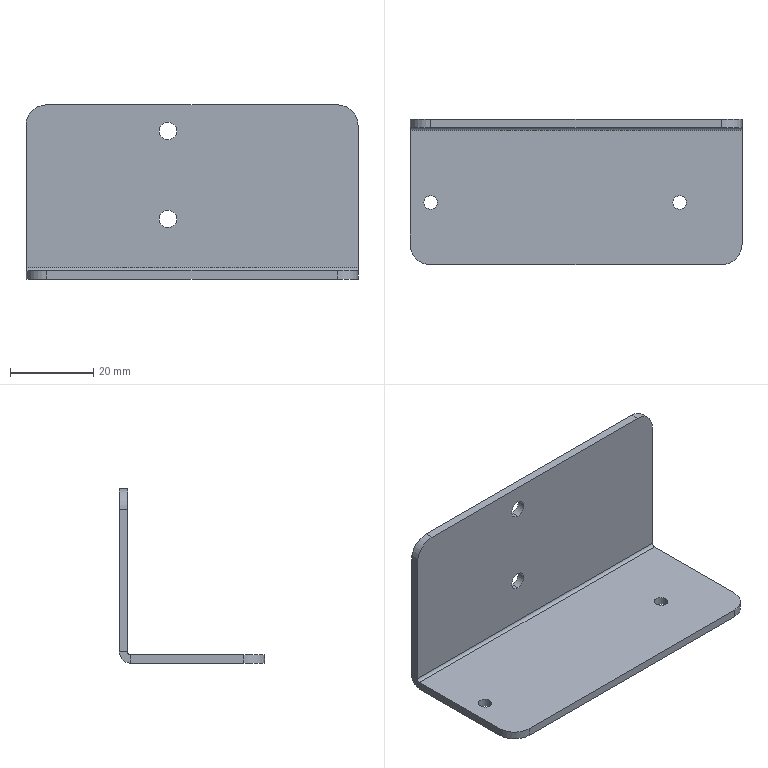Part | STEP file | H_ND24021-JJ-05-01-BJ | 1 solid | 26 faces | box 80 x 35 x 42 mm | volume 11748 mm3 | cylinder 14 | plane 12 | commonest cylinder face diameters 3.3 x4 4.2 x4 10 x4 1.473 x1 5.473 x1